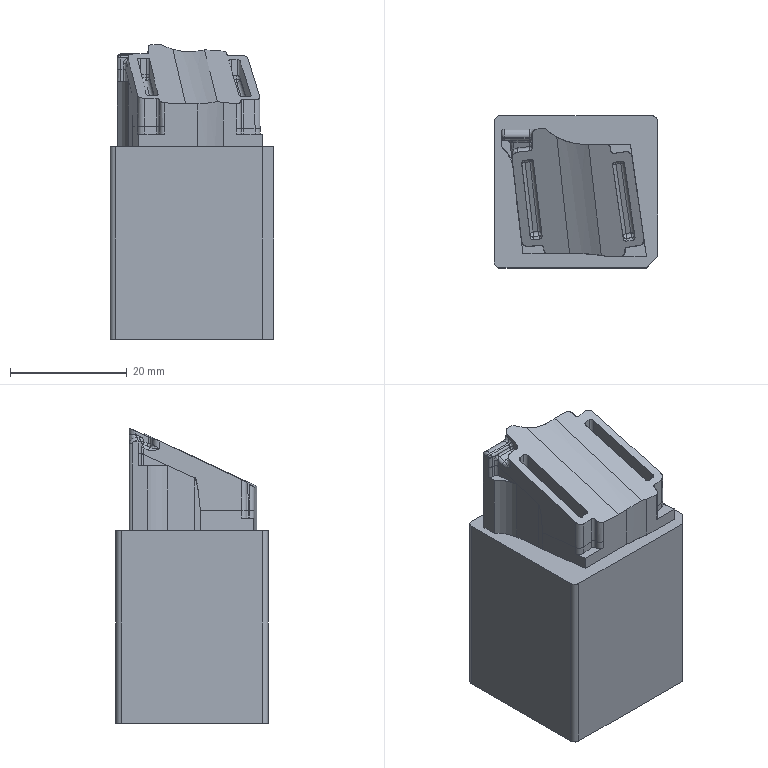NC program | NX | posted with a generic post | part box 28 x 26 x 50.455 mm
Lines 1 to 992 of 3989:
N10 G17 G21 G94 G90
(CAVITY_MILL_COPY , TOOL : 1)
N12 T00 M6
N14 G54
N16 G17 G0 G90 X-11.801 Y5.288 S0 M3
N18 G43 Z10. H0
N20 Z-1.439
N22 G94 G1 Z-1.739 F250.
N24 G3 X-12.149 Y7.314 R3.
N26 X-12.951 Y8.39 R5.56
N28 G1 X-12.962 Y8.401
N30 G3 X-12.265 Y8.115 R1.619
N32 G1 X-8.506
N34 Y7.929
N36 X-10.145 Y7.739
N38 G3 X-11.537 Y6.9 R1.933
N40 X-11.721 Y6.395 R0.983
N42 G1 X-11.829 Y6.66
N44 G3 X-12.149 Y7.314 R5.56
N46 G1 X-11.715 Y7.562
N48 X-11.746 Y7.615
N50 X-11.575
N52 X-11.685 Y7.509
N54 X-11.715 Y7.562
N56 Z-1.439
N58 G0 Z0.3
N60 X-12.199 Y4.821
N62 Z-1.786
N64 G1 Z-2.086
N66 G3 X-12.451 Y7.145 R3.
N68 X-12.899 Y7.826 R5.56
N70 G1 X-12.909 Y7.839
N72 G3 X-13.042 Y8.012 R5.56
N74 X-12.216 Y7.769 R1.525
N76 G1 X-11.889 Y7.771
N78 X-9.899 Y7.769
N80 X-10.148 Y7.74
N82 G3 X-11.924 Y5.825 R2.011
N84 X-12.451 Y7.145 R5.56
N86 G1 X-11.95 Y7.27
N88 X-11.907
N90 X-11.933 Y7.237
N92 X-11.95 Y7.27
N94 Z-1.786
N96 G0 Z-1.439
N98 X-12.303 Y4.557
N100 Z-2.134
N102 G1 Z-2.434
N104 G3 X-12.484 Y7.127 R3.
N106 X-13.053 Y7.95 R5.56
N108 X-12.265 Y7.725 R1.486
N110 G1 X-11.34
N112 X-11.171 Y7.712
N114 X-10.455 Y7.684
N116 G3 X-11.933 Y5.745 R2.027
N118 X-12.484 Y7.127 R5.56
N120 G1 X-11.968 Y7.225
N122 X-11.945
N124 X-11.958 Y7.206
N126 X-11.968 Y7.225
N128 Z-2.134
N130 G0 Z-1.786
N132 X-12.311 Y4.544
N134 Z-2.482
N136 G1 Z-2.782
N138 G3 X-12.487 Y7.125 R3.
N140 X-13.059 Y7.954 R5.56
N142 X-12.265 Y7.724 R1.495
N144 G1 X-11.788
N146 G3 X-11.23 Y7.271 R1.625
N148 X-11.936 Y5.744 R2.03
N150 X-12.487 Y7.125 R5.56
N152 G1 X-12.055 Y7.274
N154 X-11.991
N156 X-11.909 Y7.195
N158 X-11.968 Y7.11
N160 X-12.055 Y7.274
N162 Z-2.482
N164 G0 Z-2.134
N166 X-12.314 Y4.543
N168 Z-2.83
N170 G1 Z-3.13
N172 G3 X-12.489 Y7.124 R3.
N174 X-13.064 Y7.957 R5.56
N176 X-12.265 Y7.723 R1.506
N178 G1 X-12.099
N180 G3 X-11.62 Y6.866 R2.484
N182 X-11.937 Y5.737 R2.218
N184 X-12.489 Y7.124 R5.56
N186 X-14.14 Y8.492 R3.
N188 G1 Z-2.83
N190 G0 Z-2.482
N192 X-12.317 Y4.543
N194 Z-3.177
N196 G1 Z-3.477
N198 G3 X-12.49 Y7.123 R3.
N200 X-13.069 Y7.961 R5.56
N202 X-12.283 Y7.721 R1.408
N204 G1 X-12.193
N206 X-12.175 Y7.61
N208 X-11.974 Y6.791
N210 X-11.946 Y5.761
N212 G3 X-12.49 Y7.123 R5.56
N214 X-14.116 Y8.484 R3.
N216 G1 Z-3.177
N218 G0 Z-2.83
N220 X-12.32 Y4.542
N222 Z-3.525
N224 G1 Z-3.825
N226 G3 X-12.492 Y7.122 R3.
N228 X-13.069 Y7.96 R5.56
N230 X-12.436 Y7.72 R1.495
N232 G1 X-12.198
N234 X-11.975 Y5.863
N236 G3 X-12.492 Y7.122 R5.56
N238 X-14.137 Y8.491 R3.
N240 G1 Z-3.525
N242 G0 Z-3.177
N244 X-12.324 Y4.552
N246 Z-3.873
N248 G1 Z-4.173
N250 G3 X-12.482 Y7.128 R3.
N252 X-13.023 Y7.93 R5.56
N254 X-12.436 Y7.719 R1.537
N256 G1 X-12.201
N258 X-11.982 Y5.898
N260 G3 X-12.482 Y7.128 R5.56
N262 X-14.135 Y8.512 R3.
N264 G1 Z-3.873
N266 G0 Z-3.525
N268 X-12.326 Y4.542
N270 Z-4.221
N272 G1 Z-4.521
N274 G3 X-12.495 Y7.121 R3.
N276 X-13.062 Y7.948 R5.56
N278 X-12.265 Y7.719 R1.5
N280 G1 X-12.205
N282 X-12.196 Y7.638
N284 X-12.194
N286 X-11.982 Y5.868
N288 G3 X-12.495 Y7.121 R5.56
N290 X-14.127 Y8.488 R3.
N292 G1 Z-4.221
N294 G0 Z-3.873
N296 X-12.329 Y4.542
N298 Z-4.568
N300 G1 Z-4.868
N302 G3 X-12.496 Y7.12 R3.
N304 X-13.063 Y7.949 R5.56
N306 X-12.265 Y7.719 R1.5
N308 G1 X-12.205
N310 X-12.147 Y7.214
N312 X-12.135 Y7.119
N314 X-11.985 Y5.872
N316 G3 X-12.496 Y7.12 R5.56
N318 X-14.127 Y8.489 R3.
N320 G1 Z-4.568
N322 G0 Z-4.221
N324 X-12.332 Y4.542
N326 Z-4.916
N328 G1 Z-5.216
N330 G3 X-12.497 Y7.12 R3.
N332 X-13.064 Y7.949 R5.56
N334 X-12.265 Y7.719 R1.5
N336 G1 X-12.205
N338 X-12.058 Y6.452
N340 X-11.989 Y5.876
N342 G3 X-12.497 Y7.12 R5.56
N344 X-14.127 Y8.49 R3.
N346 G1 Z-4.916
N348 G0 Z-4.568
N350 X-12.336 Y4.547
N352 Z-5.264
N354 G1 Z-5.564
N356 G3 X-12.499 Y7.118 R3.
N358 X-13.065 Y7.95 R5.56
N360 X-12.265 Y7.719 R1.5
N362 G1 X-12.205
N364 X-11.989 Y5.861
N366 G3 X-12.499 Y7.118 R5.56
N368 X-14.128 Y8.492 R3.
N370 G1 Z-5.264
N372 G0 Z-4.916
N374 X-12.338 Y4.541
N376 Z-5.612
N378 G1 Z-5.912
N380 G3 X-12.499 Y7.118 R3.
N382 X-13.065 Y7.95 R5.56
N384 X-12.265 Y7.719 R1.5
N386 G1 X-12.205
N388 X-11.989 Y5.861
N390 G3 X-12.499 Y7.118 R5.56
N392 X-14.128 Y8.492 R3.
N394 G1 Z-5.612
N396 G0 Z-5.264
N398 X-12.339 Y4.538
N400 Z-5.959
N402 G1 Z-6.259
N404 G3 X-12.499 Y7.118 R3.
N406 X-13.065 Y7.95 R5.56
N408 X-12.265 Y7.719 R1.5
N410 G1 X-12.205
N412 X-11.989 Y5.861
N414 G3 X-12.499 Y7.118 R5.56
N416 X-14.128 Y8.492 R3.
N418 G1 Z-5.959
N420 G0 Z-5.612
N422 X-12.154 Y2.958
N424 Z-6.28
N426 G1 Z-6.58
N428 G3 X-12.271 Y5.518 R3.
N430 X-12.901 Y6.46 R5.56
N432 G2 X-11.845 Y4.468 R4.1
N434 G3 X-12.271 Y5.518 R5.56
N436 X-14.105 Y7. R3.
N438 G1 Z-6.28
N440 G0 Z-5.959
N442 X-12.155 Y2.954
N444 Z-6.6
N446 G1 Z-6.9
N448 G3 X-12.271 Y5.518 R3.
N450 X-12.902 Y6.461 R5.56
N452 G2 X-11.845 Y4.467 R4.1
N454 G3 X-12.271 Y5.518 R5.56
N456 X-14.105 Y7. R3.
N458 G1 Z-6.6
N460 G0 Z-6.28
N462 X-12.155 Y2.954
N464 Z-6.921
N466 G1 Z-7.221
N468 G3 X-12.271 Y5.518 R3.
N470 X-12.904 Y6.463 R5.56
N472 G2 X-11.845 Y4.467 R4.1
N474 G3 X-12.271 Y5.518 R5.56
N476 X-14.104 Y7. R3.
N478 G1 Z-6.921
N480 G0 Z-6.6
N482 X-12.155 Y2.954
N484 Z-7.269
N486 G1 Z-7.569
N488 G3 X-12.271 Y5.518 R3.
N490 X-12.905 Y6.464 R5.56
N492 G2 X-11.845 Y4.466 R4.1
N494 G3 X-12.271 Y5.518 R5.56
N496 X-14.104 Y6.999 R3.
N498 G1 Z-7.269
N500 G0 Z-6.921
N502 X-12.155 Y2.954
N504 Z-7.618
N506 G1 Z-7.918
N508 G3 X-12.272 Y5.518 R3.
N510 X-12.906 Y6.466 R5.56
N512 G2 X-11.845 Y4.465 R4.1
N514 G3 X-12.272 Y5.518 R5.56
N516 X-14.104 Y6.999 R3.
N518 G1 Z-7.618
N520 G0 Z-7.269
N522 X-12.155 Y2.954
N524 Z-7.967
N526 G1 Z-8.267
N528 G3 X-12.272 Y5.518 R3.
N530 X-12.908 Y6.467 R5.56
N532 G2 X-11.845 Y4.465 R4.1
N534 G3 X-12.272 Y5.518 R5.56
N536 X-14.104 Y6.999 R3.
N538 G1 Z-7.967
N540 G0 Z-7.618
N542 X-12.155 Y2.954
N544 Z-8.315
N546 G1 Z-8.615
N548 G3 X-12.272 Y5.518 R3.
N550 X-12.909 Y6.469 R5.56
N552 G2 X-11.845 Y4.464 R4.1
N554 G3 X-12.272 Y5.518 R5.56
N556 X-14.104 Y6.999 R3.
N558 G1 Z-8.315
N560 G0 Z-7.967
N562 X-12.155 Y2.953
N564 Z-8.664
N566 G1 Z-8.964
N568 G3 X-12.272 Y5.518 R3.
N570 X-12.911 Y6.47 R5.56
N572 G2 X-11.845 Y4.464 R4.1
N574 G3 X-12.272 Y5.518 R5.56
N576 X-14.104 Y6.999 R3.
N578 G1 Z-8.664
N580 G0 Z-8.315
N582 X-12.155 Y2.953
N584 Z-9.013
N586 G1 Z-9.313
N588 G3 X-12.272 Y5.518 R3.
N590 X-12.912 Y6.471 R5.56
N592 G2 X-11.844 Y4.463 R4.1
N594 G3 X-12.272 Y5.518 R5.56
N596 X-14.104 Y6.998 R3.
N598 G1 Z-9.013
N600 G0 Z-8.664
N602 X-12.155 Y2.953
N604 Z-9.361
N606 G1 Z-9.661
N608 G3 X-12.272 Y5.518 R3.
N610 X-12.913 Y6.473 R5.56
N612 G2 X-11.844 Y4.462 R4.1
N614 G3 X-12.272 Y5.518 R5.56
N616 X-14.104 Y6.998 R3.
N618 G1 Z-9.361
N620 G0 Z-9.013
N622 X-12.155 Y2.953
N624 Z-9.71
N626 G1 Z-10.01
N628 G3 X-12.272 Y5.517 R3.
N630 X-12.915 Y6.474 R5.56
N632 G2 X-11.844 Y4.462 R4.1
N634 G3 X-12.272 Y5.517 R5.56
N636 X-14.104 Y6.998 R3.
N638 G1 Z-9.71
N640 G0 Z-9.361
N642 X-12.155 Y2.953
N644 Z-10.059
N646 G1 Z-10.359
N648 G3 X-12.272 Y5.517 R3.
N650 X-12.916 Y6.476 R5.56
N652 G2 X-11.844 Y4.461 R4.1
N654 G3 X-12.272 Y5.517 R5.56
N656 X-14.103 Y6.998 R3.
N658 G1 Z-10.059
N660 G0 Z-9.71
N662 X-12.155 Y2.953
N664 Z-10.407
N666 G1 Z-10.707
N668 G3 X-12.272 Y5.517 R3.
N670 X-12.918 Y6.477 R5.56
N672 G2 X-11.844 Y4.461 R4.1
N674 G3 X-12.272 Y5.517 R5.56
N676 X-14.103 Y6.997 R3.
N678 G1 Z-10.407
N680 G0 Z-10.059
N682 X-12.155 Y2.953
N684 Z-10.756
N686 G1 Z-11.056
N688 G3 X-12.272 Y5.517 R3.
N690 X-12.919 Y6.479 R5.56
N692 G2 X-11.844 Y4.46 R4.1
N694 G3 X-12.272 Y5.517 R5.56
N696 X-14.103 Y6.997 R3.
N698 G1 Z-10.756
N700 G0 Z-10.407
N702 X-12.155 Y2.953
N704 Z-11.105
N706 G1 Z-11.405
N708 G3 X-12.272 Y5.517 R3.
N710 X-12.92 Y6.48 R5.56
N712 G2 X-11.844 Y4.459 R4.1
N714 G3 X-12.272 Y5.517 R5.56
N716 X-14.103 Y6.997 R3.
N718 G1 Z-11.105
N720 G0 Z-10.756
N722 X-12.155 Y2.953
N724 Z-11.453
N726 G1 Z-11.753
N728 G3 X-12.273 Y5.517 R3.
N730 X-12.922 Y6.481 R5.56
N732 G2 X-11.844 Y4.459 R4.1
N734 G3 X-12.273 Y5.517 R5.56
N736 X-14.103 Y6.997 R3.
N738 G1 Z-11.453
N740 G0 Z-11.105
N742 X-12.155 Y2.953
N744 Z-11.802
N746 G1 Z-12.102
N748 G3 X-12.273 Y5.517 R3.
N750 X-12.923 Y6.483 R5.56
N752 G2 X-11.843 Y4.458 R4.1
N754 G3 X-12.273 Y5.517 R5.56
N756 X-14.103 Y6.997 R3.
N758 G1 Z-11.802
N760 G0 Z-11.453
N762 X-12.155 Y2.953
N764 Z-12.151
N766 G1 Z-12.451
N768 G3 X-12.273 Y5.517 R3.
N770 X-12.925 Y6.484 R5.56
N772 G2 X-11.843 Y4.458 R4.1
N774 G3 X-12.273 Y5.517 R5.56
N776 X-14.103 Y6.996 R3.
N778 G1 Z-12.151
N780 G0 Z-11.802
N782 X-12.155 Y2.953
N784 Z-12.499
N786 G1 Z-12.799
N788 G3 X-12.273 Y5.517 R3.
N790 X-12.926 Y6.486 R5.56
N792 G2 X-11.843 Y4.457 R4.1
N794 G3 X-12.273 Y5.517 R5.56
N796 X-14.103 Y6.996 R3.
N798 G1 Z-12.499
N800 G0 Z-12.151
N802 X-12.155 Y2.952
N804 Z-12.848
N806 G1 Z-13.148
N808 G3 X-12.273 Y5.517 R3.
N810 X-12.927 Y6.487 R5.56
N812 G2 X-11.843 Y4.456 R4.1
N814 G3 X-12.273 Y5.517 R5.56
N816 X-14.103 Y6.996 R3.
N818 G1 Z-12.848
N820 G0 Z-12.499
N822 X-12.155 Y2.952
N824 Z-13.197
N826 G1 Z-13.497
N828 G3 X-12.273 Y5.517 R3.
N830 X-12.929 Y6.489 R5.56
N832 G2 X-11.843 Y4.456 R4.1
N834 G3 X-12.273 Y5.517 R5.56
N836 X-14.103 Y6.996 R3.
N838 G1 Z-13.197
N840 G0 Z-12.848
N842 X-12.155 Y2.952
N844 Z-13.545
N846 G1 Z-13.845
N848 G3 X-12.273 Y5.517 R3.
N850 X-12.93 Y6.49 R5.56
N852 G2 X-11.843 Y4.455 R4.1
N854 G3 X-12.273 Y5.517 R5.56
N856 X-14.102 Y6.996 R3.
N858 G1 Z-13.545
N860 G0 Z-13.197
N862 X-12.155 Y2.952
N864 Z-13.894
N866 G1 Z-14.194
N868 G3 X-12.273 Y5.517 R3.
N870 X-12.932 Y6.491 R5.56
N872 G2 X-11.843 Y4.455 R4.1
N874 G3 X-12.273 Y5.517 R5.56
N876 X-14.102 Y6.995 R3.
N878 G1 Z-13.894
N880 G0 Z-13.545
N882 X-12.155 Y2.952
N884 Z-14.243
N886 G1 Z-14.543
N888 G3 X-12.273 Y5.517 R3.
N890 X-12.933 Y6.493 R5.56
N892 G2 X-11.843 Y4.454 R4.1
N894 G3 X-12.273 Y5.517 R5.56
N896 X-14.102 Y6.995 R3.
N898 G1 Z-14.243
N900 G0 Z-13.894
N902 X-12.155 Y2.952
N904 Z-14.591
N906 G1 Z-14.891
N908 G3 X-12.273 Y5.517 R3.
N910 X-12.934 Y6.494 R5.56
N912 G2 X-11.843 Y4.454 R4.1
N914 G3 X-12.273 Y5.517 R5.56
N916 X-14.102 Y6.995 R3.
N918 G1 Z-14.591
N920 G0 Z-14.243
N922 X-12.155 Y2.952
N924 Z-14.94
N926 G1 Z-15.24
N928 G3 X-12.273 Y5.517 R3.
N930 X-12.936 Y6.496 R5.56
N932 G2 X-11.842 Y4.453 R4.1
N934 G3 X-12.273 Y5.517 R5.56
N936 X-14.102 Y6.995 R3.
N938 G1 Z-14.94
N940 G0 Z-14.591
N942 X-12.155 Y2.952
N944 Z-15.242
N946 G1 Z-15.542
N948 G3 X-12.273 Y5.517 R3.
N950 X-12.937 Y6.497 R5.56
N952 G2 X-11.842 Y4.452 R4.1
N954 G3 X-12.273 Y5.517 R5.56
N956 X-14.102 Y6.995 R3.
N958 G1 Z-15.242
N960 G0 Z-14.94
N962 X-12.155 Y2.952
N964 Z-15.544
N966 G1 Z-15.844
N968 G3 X-12.274 Y5.517 R3.
N970 X-12.938 Y6.498 R5.56
N972 G2 X-11.842 Y4.452 R4.1
N974 G3 X-12.274 Y5.517 R5.56
N976 X-14.102 Y6.994 R3.
N978 G1 Z-15.544
N980 G0 Z-15.242
N982 X-12.155 Y2.952
N984 Z-15.846
N986 G1 Z-16.146
N988 G3 X-12.274 Y5.517 R3.
N990 X-12.939 Y6.499 R5.56
N992 G2 X-11.842 Y4.451 R4.1
N994 G3 X-12.274 Y5.517 R5.56
N996 X-14.102 Y6.994 R3.
N998 G1 Z-15.846
N1000 G0 Z-15.544
N1002 X-12.155 Y2.952
N1004 Z-16.149
N1006 G1 Z-16.449
N1008 G3 X-12.274 Y5.517 R3.
N1010 X-12.941 Y6.501 R5.56
N1012 G2 X-11.842 Y4.451 R4.1
N1014 G3 X-12.274 Y5.517 R5.56
N1016 X-14.102 Y6.994 R3.
N1018 G1 Z-16.149
N1020 G0 Z-15.846
N1022 X-12.155 Y2.952
N1024 Z-16.451
N1026 G1 Z-16.751
N1028 G3 X-12.274 Y5.517 R3.
N1030 X-12.942 Y6.502 R5.56
N1032 G2 X-11.842 Y4.45 R4.1
N1034 G3 X-12.274 Y5.517 R5.56
N1036 X-14.102 Y6.994 R3.
N1038 G1 Z-16.451
N1040 G0 Z-16.149
N1042 X-12.155 Y2.951
N1044 Z-16.753
N1046 G1 Z-17.053
N1048 G3 X-12.274 Y5.517 R3.
N1050 X-12.943 Y6.503 R5.56
N1052 G2 X-11.842 Y4.45 R4.1
N1054 G3 X-12.274 Y5.517 R5.56
N1056 X-14.101 Y6.994 R3.
N1058 G1 Z-16.753
N1060 G0 Z-16.451
N1062 X-12.155 Y2.951
N1064 Z-17.055
N1066 G1 Z-17.355
N1068 G3 X-12.274 Y5.516 R3.
N1070 X-12.944 Y6.504 R5.56
N1072 G2 X-11.842 Y4.449 R4.1
N1074 G3 X-12.274 Y5.516 R5.56
N1076 X-14.101 Y6.994 R3.
N1078 G1 Z-17.055
N1080 G0 Z10.
N1082 X-6.308 Y3.845
N1084 Z-2.134
N1086 G1 Z-2.434
N1088 G3 X-8.303 Y4.238 R3.
N1090 G1 X-8.453 Y4.213
N1092 X-8.967 Y4.12
N1094 X-8.578 Y4.333
N1096 X-8.513 Y4.41
N1098 X-7.937 Y4.476
N1100 G3 X-7.632 Y4.3 R0.995
N1102 G1 X-7.717 Y4.296
N1104 G3 X-8.303 Y4.238 R5.56
N1106 X-9.941 Y3.424 R3.
N1108 G1 Z-2.134
N1110 G0 Z-1.786
N1112 X-8.719 Y2.873
N1114 Z-2.482
N1116 G1 Z-2.782
N1118 G3 X-8.25 Y4.233 R3.
N1120 X-8.251 Y4.437 R1.077
N1122 G1 X-8.196 Y4.443
N1124 G3 X-7.481 Y3.569 R1.086
N1126 G1 X-7.605 Y3.566
N1128 G3 X-8.588 Y3.453 R5.56
N1130 G1 X-8.746 Y3.42
N1132 G3 X-8.25 Y4.233 R1.077
N1134 X-8.112 Y3.026 R3.
N1136 G1 Z-2.482
N1138 G0 Z-2.134
N1140 X-7.591 Y2.812
N1142 Z-2.582
N1144 G1 X-7.6
N1146 X-8.199 Y2.77 Z-2.593
N1148 X-8.653 Y2.68 Z-2.601
N1150 X-8.437 Y2.817 Z-2.605
N1152 X-8.219 Y3.14 Z-2.612
N1154 X-8.128 Y3.518 Z-2.619
N1156 X-8.172 Y3.769 Z-2.623
N1158 X-8.224 Y4.236 Z-2.631
N1160 X-8.172 Y3.769 Z-2.64
N1162 X-8.128 Y3.518 Z-2.644
N1164 X-8.219 Y3.14 Z-2.651
N1166 X-8.437 Y2.817 Z-2.658
N1168 X-8.653 Y2.68 Z-2.662
N1170 X-8.199 Y2.77 Z-2.67
N1172 X-7.849 Y2.794 Z-2.676
N1174 X-7.6 Y2.812 Z-2.681
N1176 X-7.566 Y2.814
N1178 X-7.6 Y2.812 Z-2.682
N1180 X-8.199 Y2.77 Z-2.692
N1182 X-8.653 Y2.68 Z-2.7
N1184 X-8.437 Y2.817 Z-2.705
N1186 X-8.219 Y3.14 Z-2.712
N1188 X-8.128 Y3.518 Z-2.718
N1190 X-8.172 Y3.769 Z-2.723
N1192 X-8.224 Y4.236 Z-2.731
N1194 X-8.172 Y3.769 Z-2.739
N1196 X-8.128 Y3.518 Z-2.744
N1198 X-8.219 Y3.14 Z-2.75
N1200 X-8.437 Y2.817 Z-2.757
N1202 X-8.653 Y2.68 Z-2.762
N1204 X-8.199 Y2.77 Z-2.77
N1206 X-7.849 Y2.794 Z-2.776
N1208 X-7.6 Y2.812 Z-2.78
N1210 X-7.566 Y2.814 Z-2.781
N1212 X-7.6 Y2.812
N1214 X-8.199 Y2.77 Z-2.792
N1216 X-8.653 Y2.68 Z-2.8
N1218 X-8.437 Y2.817 Z-2.804
N1220 X-8.219 Y3.14 Z-2.811
N1222 X-8.128 Y3.518 Z-2.818
N1224 X-8.172 Y3.769 Z-2.822
N1226 X-8.224 Y4.236 Z-2.831
N1228 X-8.172 Y3.769 Z-2.839
N1230 X-8.128 Y3.518 Z-2.843
N1232 X-8.219 Y3.14 Z-2.85
N1234 X-8.437 Y2.817 Z-2.857
N1236 X-8.653 Y2.68 Z-2.861
N1238 X-8.199 Y2.77 Z-2.869
N1240 X-7.849 Y2.794 Z-2.876
N1242 X-7.6 Y2.812 Z-2.88
N1244 X-7.566 Y2.814 Z-2.881
N1246 X-7.6 Y2.812
N1248 X-8.199 Y2.77 Z-2.892
N1250 X-8.653 Y2.68 Z-2.9
N1252 X-8.437 Y2.817 Z-2.904
N1254 X-8.219 Y3.14 Z-2.911
N1256 X-8.128 Y3.518 Z-2.918
N1258 X-8.172 Y3.769 Z-2.922
N1260 X-8.224 Y4.236 Z-2.93
N1262 X-8.172 Y3.769 Z-2.939
N1264 X-8.128 Y3.518 Z-2.943
N1266 X-8.219 Y3.14 Z-2.95
N1268 X-8.437 Y2.817 Z-2.957
N1270 X-8.653 Y2.68 Z-2.961
N1272 X-8.199 Y2.77 Z-2.969
N1274 X-7.849 Y2.794 Z-2.975
N1276 X-7.6 Y2.812 Z-2.98
N1278 X-7.566 Y2.814
N1280 X-7.6 Y2.812 Z-2.981
N1282 X-8.199 Y2.77 Z-2.991
N1284 X-8.653 Y2.68 Z-2.999
N1286 X-8.437 Y2.817 Z-3.004
N1288 X-8.219 Y3.14 Z-3.011
N1290 X-8.128 Y3.518 Z-3.017
N1292 X-8.172 Y3.769 Z-3.022
N1294 X-8.224 Y4.236 Z-3.03
N1296 X-8.172 Y3.769 Z-3.038
N1298 X-8.128 Y3.518 Z-3.043
N1300 X-8.219 Y3.14 Z-3.049
N1302 X-8.437 Y2.817 Z-3.056
N1304 X-8.653 Y2.68 Z-3.061
N1306 X-8.199 Y2.77 Z-3.069
N1308 X-7.849 Y2.794 Z-3.075
N1310 X-7.6 Y2.812 Z-3.079
N1312 X-7.566 Y2.814 Z-3.08
N1314 X-7.6 Y2.812
N1316 X-8.199 Y2.77 Z-3.091
N1318 X-8.653 Y2.68 Z-3.099
N1320 X-8.437 Y2.817 Z-3.103
N1322 X-8.219 Y3.14 Z-3.11
N1324 X-8.128 Y3.518 Z-3.117
N1326 X-8.172 Y3.769 Z-3.121
N1328 X-8.224 Y4.236 Z-3.13
N1330 X-8.247 Y4.434
N1332 X-8.201 Y4.44
N1334 X-8.123 Y3.777
N1336 G3 X-7.393 Y2.821 R1.07
N1338 G1 X-7.409 Y2.82
N1340 G3 X-7.633 Y2.809 R5.56
N1342 G1 X-7.849 Y2.794
N1344 G3 X-8.543 Y2.702 R5.56
N1346 G1 X-8.653 Y2.68
N1348 G3 X-8.172 Y3.769 R1.069
N1350 G1 X-8.224 Y4.236
N1352 Z-2.83
N1354 G0 Z-2.482
N1356 X-8.276 Y1.985
N1358 Z-2.93
N1360 G1 X-8.369 Y1.972 Z-2.931
N1362 X-8.476 Y1.952 Z-2.933
N1364 X-8.588 Y1.931 Z-2.935
N1366 X-8.369 Y2.065 Z-2.94
N1368 X-8.142 Y2.391 Z-2.947
N1370 X-8.044 Y2.776 Z-2.954
N1372 X-8.086 Y3.029 Z-2.958
N1374 X-8.221 Y4.236 Z-2.979
N1376 X-8.086 Y3.029 Z-3.
N1378 X-8.044 Y2.776 Z-3.005
N1380 X-8.142 Y2.391 Z-3.012
N1382 X-8.369 Y2.065 Z-3.019
N1384 X-8.588 Y1.931 Z-3.023
N1386 X-8.476 Y1.952 Z-3.025
N1388 X-8.369 Y1.972 Z-3.027
N1390 X-8.261 Y1.987 Z-3.029
N1392 X-8.369 Y1.972 Z-3.031
N1394 X-8.476 Y1.952 Z-3.033
N1396 X-8.588 Y1.931 Z-3.035
N1398 X-8.369 Y2.065 Z-3.039
N1400 X-8.142 Y2.391 Z-3.046
N1402 X-8.044 Y2.776 Z-3.053
N1404 X-8.086 Y3.029 Z-3.058
N1406 X-8.221 Y4.236 Z-3.079
N1408 X-8.086 Y3.029 Z-3.1
N1410 X-8.044 Y2.776 Z-3.105
N1412 X-8.142 Y2.391 Z-3.111
N1414 X-8.369 Y2.065 Z-3.118
N1416 X-8.588 Y1.931 Z-3.123
N1418 X-8.476 Y1.952 Z-3.125
N1420 X-8.369 Y1.972 Z-3.127
N1422 X-8.261 Y1.987 Z-3.129
N1424 X-8.369 Y1.972 Z-3.131
N1426 X-8.476 Y1.952 Z-3.132
N1428 X-8.588 Y1.931 Z-3.134
N1430 X-8.369 Y2.065 Z-3.139
N1432 X-8.142 Y2.391 Z-3.146
N1434 X-8.044 Y2.776 Z-3.153
N1436 X-8.086 Y3.029 Z-3.157
N1438 X-8.221 Y4.236 Z-3.179
N1440 X-8.086 Y3.029 Z-3.2
N1442 X-8.044 Y2.776 Z-3.204
N1444 X-8.142 Y2.391 Z-3.211
N1446 X-8.369 Y2.065 Z-3.218
N1448 X-8.588 Y1.931 Z-3.223
N1450 X-8.476 Y1.952 Z-3.225
N1452 X-8.369 Y1.972 Z-3.226
N1454 X-8.261 Y1.987 Z-3.228
N1456 X-8.369 Y1.972 Z-3.23
N1458 X-8.476 Y1.952 Z-3.232
N1460 X-8.588 Y1.931 Z-3.234
N1462 X-8.369 Y2.065 Z-3.239
N1464 X-8.142 Y2.391 Z-3.246
N1466 X-8.044 Y2.776 Z-3.252
N1468 X-8.086 Y3.029 Z-3.257
N1470 X-8.221 Y4.236 Z-3.278
N1472 X-8.086 Y3.029 Z-3.299
N1474 X-8.044 Y2.776 Z-3.304
N1476 X-8.142 Y2.391 Z-3.311
N1478 X-8.369 Y2.065 Z-3.318
N1480 X-8.588 Y1.931 Z-3.322
N1482 X-8.476 Y1.952 Z-3.324
N1484 X-8.369 Y1.972 Z-3.326
N1486 X-8.261 Y1.987 Z-3.328
N1488 X-8.369 Y1.972 Z-3.33
N1490 X-8.476 Y1.952 Z-3.332
N1492 X-8.588 Y1.931 Z-3.334
N1494 X-8.369 Y2.065 Z-3.338
N1496 X-8.142 Y2.391 Z-3.345
N1498 X-8.044 Y2.776 Z-3.352
N1500 X-8.086 Y3.029 Z-3.357
N1502 X-8.221 Y4.236 Z-3.378
N1504 X-8.086 Y3.029 Z-3.399
N1506 X-8.044 Y2.776 Z-3.403
N1508 X-8.142 Y2.391 Z-3.41
N1510 X-8.369 Y2.065 Z-3.417
N1512 X-8.588 Y1.931 Z-3.422
N1514 X-8.476 Y1.952 Z-3.424
N1516 X-8.369 Y1.972 Z-3.426
N1518 X-8.261 Y1.987 Z-3.428
N1520 X-8.369 Y1.972 Z-3.429
N1522 X-8.476 Y1.952 Z-3.431
N1524 X-8.588 Y1.931 Z-3.433
N1526 X-8.369 Y2.065 Z-3.438
N1528 X-8.142 Y2.391 Z-3.445
N1530 X-8.044 Y2.776 Z-3.452
N1532 X-8.086 Y3.029 Z-3.456
N1534 X-8.221 Y4.236 Z-3.477
N1536 X-8.243 Y4.432
N1538 X-8.203 Y4.437
N1540 X-8.037 Y3.037
N1542 G3 X-7.29 Y2.075 R1.07
N1544 X-7.494 Y2.061 R5.56
N1546 G1 X-7.925 Y2.025
N1548 G3 X-8.476 Y1.952 R5.56
N1550 G1 X-8.588 Y1.931
N1552 G3 X-8.086 Y3.029 R1.079
N1554 G1 X-8.221 Y4.236
N1556 Z-3.177
N1558 G0 Z-2.482
N1560 X-8.151 Y1.54
N1562 Z-3.277
N1564 G1 X-8.204 Y1.468 Z-3.279
N1566 X-8.051 Y1.675 Z-3.283
N1568 X-7.964 Y2.013 Z-3.29
N1570 X-7.999 Y2.268 Z-3.294
N1572 X-8.013 Y2.399 Z-3.296
N1574 X-8.218 Y4.237 Z-3.329
N1576 X-8.013 Y2.399 Z-3.361
N1578 X-7.999 Y2.268 Z-3.363
N1580 X-7.964 Y2.013 Z-3.368
N1582 X-8.051 Y1.675 Z-3.374
N1584 X-8.204 Y1.468 Z-3.378
N1586 X-8.051 Y1.675 Z-3.383
N1588 X-7.964 Y2.013 Z-3.389
N1590 X-7.999 Y2.268 Z-3.393
N1592 X-8.013 Y2.399 Z-3.396
N1594 X-8.218 Y4.237 Z-3.428
N1596 X-8.013 Y2.399 Z-3.46
N1598 X-7.999 Y2.268 Z-3.463
N1600 X-7.964 Y2.013 Z-3.467
N1602 X-8.051 Y1.675 Z-3.473
N1604 X-8.204 Y1.468 Z-3.478
N1606 X-8.051 Y1.675 Z-3.482
N1608 X-7.964 Y2.013 Z-3.488
N1610 X-7.999 Y2.268 Z-3.493
N1612 X-8.013 Y2.399 Z-3.495
N1614 X-8.218 Y4.237 Z-3.527
N1616 X-8.013 Y2.399 Z-3.56
N1618 X-7.999 Y2.268 Z-3.562
N1620 X-7.964 Y2.013 Z-3.566
N1622 X-8.051 Y1.675 Z-3.572
N1624 X-8.204 Y1.468 Z-3.577
N1626 X-8.051 Y1.675 Z-3.581
N1628 X-7.964 Y2.013 Z-3.587
N1630 X-7.999 Y2.268 Z-3.592
N1632 X-8.013 Y2.399 Z-3.594
N1634 X-8.218 Y4.237 Z-3.627
N1636 X-8.013 Y2.399 Z-3.659
N1638 X-7.999 Y2.268 Z-3.661
N1640 X-7.964 Y2.013 Z-3.666
N1642 X-8.051 Y1.675 Z-3.672
N1644 X-8.204 Y1.468 Z-3.676
N1646 X-8.051 Y1.675 Z-3.681
N1648 X-7.964 Y2.013 Z-3.687
N1650 X-7.999 Y2.268 Z-3.691
N1652 X-8.013 Y2.399 Z-3.694
N1654 X-8.218 Y4.237 Z-3.726
N1656 X-8.013 Y2.399 Z-3.758
N1658 X-7.999 Y2.268 Z-3.76
N1660 X-7.964 Y2.013 Z-3.765
N1662 X-8.051 Y1.675 Z-3.771
N1664 X-8.204 Y1.468 Z-3.776
N1666 X-8.051 Y1.675 Z-3.78
N1668 X-7.964 Y2.013 Z-3.786
N1670 X-7.999 Y2.268 Z-3.791
N1672 X-8.013 Y2.399 Z-3.793
N1674 X-8.218 Y4.237 Z-3.825
N1676 X-8.24 Y4.429
N1678 X-8.204 Y4.433
N1680 X-7.951 Y2.296
N1682 G3 X-7.215 Y1.338 R1.07
N1684 X-7.778 Y1.291 R5.56
N1686 G1 X-8.207 Y1.233
N1688 G3 X-8.438 Y1.197 R5.56
N1690 G1 X-8.521 Y1.182
N1692 G3 X-7.999 Y2.268 R1.091
N1694 G1 X-8.013 Y2.399
N1696 X-8.218 Y4.237
N1698 Z-3.525
N1700 G0 Z-3.177
N1702 X-7.932 Y1.702
N1704 Z-3.625
N1706 G1 X-7.914 Y1.548 Z-3.628
N1708 X-7.904 Y1.488 Z-3.629
N1710 X-7.9 Y1.427 Z-3.63
N1712 X-7.904 Y1.488 Z-3.631
N1714 X-7.914 Y1.548 Z-3.632
N1716 X-8.215 Y4.237 Z-3.679
N1718 X-7.914 Y1.548 Z-3.727
N1720 X-7.904 Y1.488 Z-3.728
N1722 X-7.9 Y1.427 Z-3.729
N1724 X-7.904 Y1.488 Z-3.73
N1726 X-7.914 Y1.548 Z-3.731
N1728 X-8.215 Y4.237 Z-3.778
N1730 X-7.914 Y1.548 Z-3.825
N1732 X-7.904 Y1.488 Z-3.826
N1734 X-7.9 Y1.427 Z-3.827
N1736 X-7.904 Y1.488 Z-3.828
N1738 X-7.914 Y1.548 Z-3.83
N1740 X-8.215 Y4.237 Z-3.877
N1742 X-7.914 Y1.548 Z-3.924
N1744 X-7.904 Y1.488 Z-3.925
N1746 X-7.9 Y1.427 Z-3.926
N1748 X-7.904 Y1.488 Z-3.927
N1750 X-7.914 Y1.548 Z-3.928
N1752 X-8.215 Y4.237 Z-3.975
N1754 X-7.914 Y1.548 Z-4.023
N1756 X-7.904 Y1.488 Z-4.024
N1758 X-7.9 Y1.427 Z-4.025
N1760 X-7.904 Y1.488 Z-4.026
N1762 X-7.914 Y1.548 Z-4.027
N1764 X-8.215 Y4.237 Z-4.074
N1766 X-7.914 Y1.548 Z-4.121
N1768 X-7.904 Y1.488 Z-4.122
N1770 X-7.9 Y1.427 Z-4.124
N1772 X-7.904 Y1.488 Z-4.125
N1774 X-7.914 Y1.548 Z-4.126
N1776 X-8.215 Y4.237 Z-4.173
N1778 X-8.237 Y4.426
N1780 X-8.206 Y4.43
N1782 X-7.865 Y1.556
N1784 G3 X-7.141 Y0.601 R1.07
N1786 X-7.758 Y0.555 R5.56
N1788 G1 X-7.973 Y0.527
N1790 G3 X-8.403 Y0.453 R5.56
N1792 X-7.914 Y1.548 R1.069
N1794 G1 X-8.215 Y4.237
N1796 Z-3.873
N1798 G0 Z-3.525
N1800 X-7.929 Y1.704
N1802 Z-3.973
N1804 G1 X-7.898 Y1.427 Z-3.978
N1806 X-8.212 Y4.237 Z-4.027
N1808 X-7.898 Y1.427 Z-4.076
N1810 X-8.212 Y4.237 Z-4.126
N1812 X-7.898 Y1.427 Z-4.175
N1814 X-8.212 Y4.237 Z-4.225
N1816 X-7.898 Y1.427 Z-4.274
N1818 X-8.212 Y4.237 Z-4.323
N1820 X-7.898 Y1.427 Z-4.373
N1822 X-8.212 Y4.237 Z-4.422
N1824 X-7.898 Y1.427 Z-4.471
N1826 X-8.212 Y4.237 Z-4.521
N1828 X-8.233 Y4.424
N1830 X-8.207 Y4.427
N1832 X-7.779 Y0.815
N1834 G3 X-6.952 Y-0.169 R1.07
N1836 G1 X-8.409 Y-0.338
N1838 G3 X-7.828 Y0.807 R1.069
N1840 G1 X-8.212 Y4.237
N1842 Z-4.221
N1844 G0 Z-3.873
N1846 X-7.926 Y1.704
N1848 Z-4.321
N1850 G1 X-7.895 Y1.428 Z-4.326
N1852 X-8.209 Y4.238 Z-4.375
N1854 X-7.895 Y1.428 Z-4.424
N1856 X-8.209 Y4.238 Z-4.474
N1858 X-7.895 Y1.428 Z-4.523
N1860 X-8.209 Y4.238 Z-4.572
N1862 X-7.895 Y1.428 Z-4.622
N1864 X-8.209 Y4.238 Z-4.671
N1866 X-7.895 Y1.428 Z-4.72
N1868 X-8.209 Y4.238 Z-4.77
N1870 X-7.895 Y1.428 Z-4.819
N1872 X-8.209 Y4.238 Z-4.868
N1874 X-8.23 Y4.419
N1876 X-8.208 Y4.422
N1878 X-7.693 Y0.075
N1880 G3 X-6.963 Y-0.882 R1.07
N1882 X-7.205 Y-0.894 R5.56
N1884 G1 X-7.423 Y-0.909
N1886 G3 X-8.226 Y-1.024 R5.56
N1888 X-7.743 Y0.067 R1.069
N1890 G1 X-8.209 Y4.238
N1892 Z-4.568
N1894 G0 Z-4.221
N1896 X-7.923 Y1.705
N1898 Z-4.668
N1900 G1 X-7.892 Y1.428 Z-4.673
N1902 X-8.206 Y4.238 Z-4.723
N1904 X-7.892 Y1.428 Z-4.772
N1906 X-8.206 Y4.238 Z-4.821
N1908 X-7.892 Y1.428 Z-4.871
N1910 X-8.206 Y4.238 Z-4.92
N1912 X-7.892 Y1.428 Z-4.969
N1914 X-8.206 Y4.238 Z-5.019
N1916 X-7.892 Y1.428 Z-5.068
N1918 X-8.206 Y4.238 Z-5.117
N1920 X-7.892 Y1.428 Z-5.167
N1922 X-8.206 Y4.238 Z-5.216
N1924 X-8.208 Y4.252
N1926 X-8.214 Y4.333
N1928 X-8.224 Y4.42
N1930 X-8.21 Y4.421
N1932 X-7.607 Y-0.666
N1934 G3 X-6.878 Y-1.622 R1.07
N1936 X-7.191 Y-1.639 R5.56
N1938 G1 X-7.409 Y-1.657
N1940 G3 X-8.141 Y-1.766 R5.56
N1942 X-7.657 Y-0.674 R1.069
N1944 G1 X-8.206 Y4.238
N1946 Z-4.916
N1948 G0 Z-4.568
N1950 X-7.92 Y1.705
N1952 Z-5.016
N1954 G1 X-7.889 Y1.428 Z-5.021
N1956 X-8.196 Y4.169 Z-5.069
N1958 X-8.203 Y4.238 Z-5.07
N1960 X-8.196 Y4.169 Z-5.072
N1962 X-7.889 Y1.428 Z-5.12
N1964 X-8.196 Y4.169 Z-5.168
N1966 X-8.203 Y4.238 Z-5.169
N1968 X-8.196 Y4.169 Z-5.17
N1970 X-7.889 Y1.428 Z-5.218
N1972 X-8.196 Y4.169 Z-5.267
N1974 X-8.203 Y4.238 Z-5.268
N1976 X-8.196 Y4.169 Z-5.269
N1978 X-7.889 Y1.428 Z-5.317
N1980 X-8.196 Y4.169 Z-5.365
N1982 X-8.203 Y4.238 Z-5.366